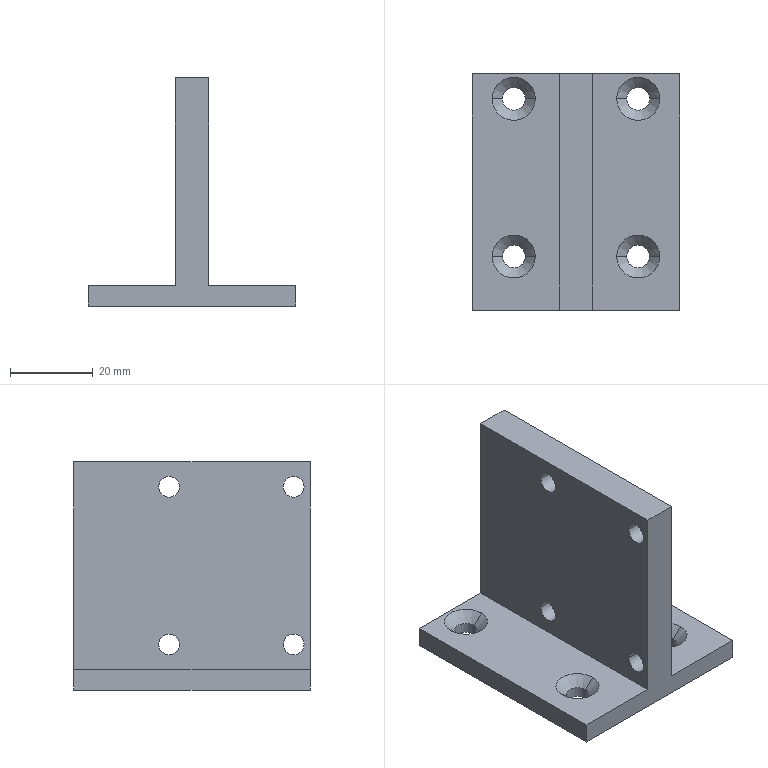Part | 1 solid | 34 faces | box 50 x 57 x 55 mm | volume 35677 mm3 | cylinder 16 | plane 10 | cone 8 | commonest cylinder face diameters 5 x8 5.5 x8
STEP:
#1=CARTESIAN_POINT('',(7.25,41.,2.55));
#2=VERTEX_POINT('',#1);
#3=CARTESIAN_POINT('',(12.75,41.,2.55));
#4=VERTEX_POINT('',#3);
#5=CARTESIAN_POINT('',(10.,41.,2.55));
#6=DIRECTION('',(0.,0.,1.));
#7=DIRECTION('',(1.,0.,0.));
#8=AXIS2_PLACEMENT_3D('',#5,#6,#7);
#9=CIRCLE('',#8,2.75);
#10=EDGE_CURVE('',#2,#4,#9,.T.);
#11=ORIENTED_EDGE('',*,*,#10,.F.);
#12=CARTESIAN_POINT('',(4.8,41.,5.));
#13=VERTEX_POINT('',#12);
#14=CARTESIAN_POINT('',(4.8,41.,5.));
#15=DIRECTION('',(-0.7071,0.,0.7071));
#16=VECTOR('',#15,1000.);
#17=LINE('',#14,#16);
#18=EDGE_CURVE('',#2,#13,#17,.T.);
#19=ORIENTED_EDGE('',*,*,#18,.T.);
#20=CARTESIAN_POINT('',(15.2,41.,5.));
#21=VERTEX_POINT('',#20);
#22=CARTESIAN_POINT('',(10.,41.,5.));
#23=DIRECTION('',(0.,0.,1.));
#24=DIRECTION('',(1.,0.,0.));
#25=AXIS2_PLACEMENT_3D('',#22,#23,#24);
#26=CIRCLE('',#25,5.2);
#27=EDGE_CURVE('',#13,#21,#26,.T.);
#28=ORIENTED_EDGE('',*,*,#27,.T.);
#29=CARTESIAN_POINT('',(15.2,41.,5.));
#30=DIRECTION('',(0.7071,0.,0.7071));
#31=VECTOR('',#30,1000.);
#32=LINE('',#29,#31);
#33=EDGE_CURVE('',#4,#21,#32,.T.);
#34=ORIENTED_EDGE('',*,*,#33,.F.);
#35=EDGE_LOOP('',(#11,#19,#28,#34));
#36=FACE_OUTER_BOUND('',#35,.T.);
#37=CARTESIAN_POINT('',(10.,41.,5.));
#38=DIRECTION('',(0.,0.,1.));
#39=DIRECTION('',(1.,0.,0.));
#40=AXIS2_PLACEMENT_3D('',#37,#38,#39);
#41=CONICAL_SURFACE('',#40,5.2,0.7854);
#42=ADVANCED_FACE('',(#36),#41,.F.);
#43=CARTESIAN_POINT('',(7.25,41.,0.));
#44=VERTEX_POINT('',#43);
#45=CARTESIAN_POINT('',(12.75,41.,0.));
#46=VERTEX_POINT('',#45);
#47=CARTESIAN_POINT('',(10.,41.,0.));
#48=DIRECTION('',(0.,0.,1.));
#49=DIRECTION('',(1.,0.,0.));
#50=AXIS2_PLACEMENT_3D('',#47,#48,#49);
#51=CIRCLE('',#50,2.75);
#52=EDGE_CURVE('',#44,#46,#51,.T.);
#53=ORIENTED_EDGE('',*,*,#52,.F.);
#54=CARTESIAN_POINT('',(7.25,41.,5.));
#55=DIRECTION('',(0.,0.,1.));
#56=VECTOR('',#55,1000.);
#57=LINE('',#54,#56);
#58=EDGE_CURVE('',#44,#2,#57,.T.);
#59=ORIENTED_EDGE('',*,*,#58,.T.);
#60=ORIENTED_EDGE('',*,*,#10,.T.);
#61=CARTESIAN_POINT('',(12.75,41.,5.));
#62=DIRECTION('',(0.,0.,1.));
#63=VECTOR('',#62,1000.);
#64=LINE('',#61,#63);
#65=EDGE_CURVE('',#46,#4,#64,.T.);
#66=ORIENTED_EDGE('',*,*,#65,.F.);
#67=EDGE_LOOP('',(#53,#59,#60,#66));
#68=FACE_OUTER_BOUND('',#67,.T.);
#69=CARTESIAN_POINT('',(10.,41.,5.));
#70=DIRECTION('',(0.,0.,1.));
#71=DIRECTION('',(1.,0.,0.));
#72=AXIS2_PLACEMENT_3D('',#69,#70,#71);
#73=CYLINDRICAL_SURFACE('',#72,2.75);
#74=ADVANCED_FACE('',(#68),#73,.F.);
#75=CARTESIAN_POINT('',(7.25,3.,2.55));
#76=VERTEX_POINT('',#75);
#77=CARTESIAN_POINT('',(12.75,3.,2.55));
#78=VERTEX_POINT('',#77);
#79=CARTESIAN_POINT('',(10.,3.,2.55));
#80=DIRECTION('',(0.,0.,1.));
#81=DIRECTION('',(1.,0.,0.));
#82=AXIS2_PLACEMENT_3D('',#79,#80,#81);
#83=CIRCLE('',#82,2.75);
#84=EDGE_CURVE('',#76,#78,#83,.T.);
#85=ORIENTED_EDGE('',*,*,#84,.F.);
#86=CARTESIAN_POINT('',(4.8,3.,5.));
#87=VERTEX_POINT('',#86);
#88=CARTESIAN_POINT('',(4.8,3.,5.));
#89=DIRECTION('',(-0.7071,0.,0.7071));
#90=VECTOR('',#89,1000.);
#91=LINE('',#88,#90);
#92=EDGE_CURVE('',#76,#87,#91,.T.);
#93=ORIENTED_EDGE('',*,*,#92,.T.);
#94=CARTESIAN_POINT('',(15.2,3.,5.));
#95=VERTEX_POINT('',#94);
#96=CARTESIAN_POINT('',(10.,3.,5.));
#97=DIRECTION('',(0.,0.,1.));
#98=DIRECTION('',(1.,0.,0.));
#99=AXIS2_PLACEMENT_3D('',#96,#97,#98);
#100=CIRCLE('',#99,5.2);
#101=EDGE_CURVE('',#87,#95,#100,.T.);
#102=ORIENTED_EDGE('',*,*,#101,.T.);
#103=CARTESIAN_POINT('',(15.2,3.,5.));
#104=DIRECTION('',(0.7071,0.,0.7071));
#105=VECTOR('',#104,1000.);
#106=LINE('',#103,#105);
#107=EDGE_CURVE('',#78,#95,#106,.T.);
#108=ORIENTED_EDGE('',*,*,#107,.F.);
#109=EDGE_LOOP('',(#85,#93,#102,#108));
#110=FACE_OUTER_BOUND('',#109,.T.);
#111=CARTESIAN_POINT('',(10.,3.,5.));
#112=DIRECTION('',(0.,0.,1.));
#113=DIRECTION('',(1.,0.,0.));
#114=AXIS2_PLACEMENT_3D('',#111,#112,#113);
#115=CONICAL_SURFACE('',#114,5.2,0.7854);
#116=ADVANCED_FACE('',(#110),#115,.F.);
#117=CARTESIAN_POINT('',(7.25,3.,0.));
#118=VERTEX_POINT('',#117);
#119=CARTESIAN_POINT('',(12.75,3.,0.));
#120=VERTEX_POINT('',#119);
#121=CARTESIAN_POINT('',(10.,3.,0.));
#122=DIRECTION('',(0.,0.,1.));
#123=DIRECTION('',(1.,0.,0.));
#124=AXIS2_PLACEMENT_3D('',#121,#122,#123);
#125=CIRCLE('',#124,2.75);
#126=EDGE_CURVE('',#118,#120,#125,.T.);
#127=ORIENTED_EDGE('',*,*,#126,.F.);
#128=CARTESIAN_POINT('',(7.25,3.,5.));
#129=DIRECTION('',(0.,0.,1.));
#130=VECTOR('',#129,1000.);
#131=LINE('',#128,#130);
#132=EDGE_CURVE('',#118,#76,#131,.T.);
#133=ORIENTED_EDGE('',*,*,#132,.T.);
#134=ORIENTED_EDGE('',*,*,#84,.T.);
#135=CARTESIAN_POINT('',(12.75,3.,5.));
#136=DIRECTION('',(0.,0.,1.));
#137=VECTOR('',#136,1000.);
#138=LINE('',#135,#137);
#139=EDGE_CURVE('',#120,#78,#138,.T.);
#140=ORIENTED_EDGE('',*,*,#139,.F.);
#141=EDGE_LOOP('',(#127,#133,#134,#140));
#142=FACE_OUTER_BOUND('',#141,.T.);
#143=CARTESIAN_POINT('',(10.,3.,5.));
#144=DIRECTION('',(0.,0.,1.));
#145=DIRECTION('',(1.,0.,0.));
#146=AXIS2_PLACEMENT_3D('',#143,#144,#145);
#147=CYLINDRICAL_SURFACE('',#146,2.75);
#148=ADVANCED_FACE('',(#142),#147,.F.);
#149=CARTESIAN_POINT('',(37.25,41.,2.55));
#150=VERTEX_POINT('',#149);
#151=CARTESIAN_POINT('',(42.75,41.,2.55));
#152=VERTEX_POINT('',#151);
#153=CARTESIAN_POINT('',(40.,41.,2.55));
#154=DIRECTION('',(0.,0.,1.));
#155=DIRECTION('',(1.,0.,0.));
#156=AXIS2_PLACEMENT_3D('',#153,#154,#155);
#157=CIRCLE('',#156,2.75);
#158=EDGE_CURVE('',#150,#152,#157,.T.);
#159=ORIENTED_EDGE('',*,*,#158,.F.);
#160=CARTESIAN_POINT('',(34.8,41.,5.));
#161=VERTEX_POINT('',#160);
#162=CARTESIAN_POINT('',(34.8,41.,5.));
#163=DIRECTION('',(-0.7071,0.,0.7071));
#164=VECTOR('',#163,1000.);
#165=LINE('',#162,#164);
#166=EDGE_CURVE('',#150,#161,#165,.T.);
#167=ORIENTED_EDGE('',*,*,#166,.T.);
#168=CARTESIAN_POINT('',(45.2,41.,5.));
#169=VERTEX_POINT('',#168);
#170=CARTESIAN_POINT('',(40.,41.,5.));
#171=DIRECTION('',(0.,0.,1.));
#172=DIRECTION('',(1.,0.,0.));
#173=AXIS2_PLACEMENT_3D('',#170,#171,#172);
#174=CIRCLE('',#173,5.2);
#175=EDGE_CURVE('',#161,#169,#174,.T.);
#176=ORIENTED_EDGE('',*,*,#175,.T.);
#177=CARTESIAN_POINT('',(45.2,41.,5.));
#178=DIRECTION('',(0.7071,0.,0.7071));
#179=VECTOR('',#178,1000.);
#180=LINE('',#177,#179);
#181=EDGE_CURVE('',#152,#169,#180,.T.);
#182=ORIENTED_EDGE('',*,*,#181,.F.);
#183=EDGE_LOOP('',(#159,#167,#176,#182));
#184=FACE_OUTER_BOUND('',#183,.T.);
#185=CARTESIAN_POINT('',(40.,41.,5.));
#186=DIRECTION('',(0.,0.,1.));
#187=DIRECTION('',(1.,0.,0.));
#188=AXIS2_PLACEMENT_3D('',#185,#186,#187);
#189=CONICAL_SURFACE('',#188,5.2,0.7854);
#190=ADVANCED_FACE('',(#184),#189,.F.);
#191=CARTESIAN_POINT('',(37.25,41.,0.));
#192=VERTEX_POINT('',#191);
#193=CARTESIAN_POINT('',(42.75,41.,0.));
#194=VERTEX_POINT('',#193);
#195=CARTESIAN_POINT('',(40.,41.,0.));
#196=DIRECTION('',(0.,0.,1.));
#197=DIRECTION('',(1.,0.,0.));
#198=AXIS2_PLACEMENT_3D('',#195,#196,#197);
#199=CIRCLE('',#198,2.75);
#200=EDGE_CURVE('',#192,#194,#199,.T.);
#201=ORIENTED_EDGE('',*,*,#200,.F.);
#202=CARTESIAN_POINT('',(37.25,41.,5.));
#203=DIRECTION('',(0.,0.,1.));
#204=VECTOR('',#203,1000.);
#205=LINE('',#202,#204);
#206=EDGE_CURVE('',#192,#150,#205,.T.);
#207=ORIENTED_EDGE('',*,*,#206,.T.);
#208=ORIENTED_EDGE('',*,*,#158,.T.);
#209=CARTESIAN_POINT('',(42.75,41.,5.));
#210=DIRECTION('',(0.,0.,1.));
#211=VECTOR('',#210,1000.);
#212=LINE('',#209,#211);
#213=EDGE_CURVE('',#194,#152,#212,.T.);
#214=ORIENTED_EDGE('',*,*,#213,.F.);
#215=EDGE_LOOP('',(#201,#207,#208,#214));
#216=FACE_OUTER_BOUND('',#215,.T.);
#217=CARTESIAN_POINT('',(40.,41.,5.));
#218=DIRECTION('',(0.,0.,1.));
#219=DIRECTION('',(1.,0.,0.));
#220=AXIS2_PLACEMENT_3D('',#217,#218,#219);
#221=CYLINDRICAL_SURFACE('',#220,2.75);
#222=ADVANCED_FACE('',(#216),#221,.F.);
#223=CARTESIAN_POINT('',(37.25,3.,2.55));
#224=VERTEX_POINT('',#223);
#225=CARTESIAN_POINT('',(42.75,3.,2.55));
#226=VERTEX_POINT('',#225);
#227=CARTESIAN_POINT('',(40.,3.,2.55));
#228=DIRECTION('',(0.,0.,1.));
#229=DIRECTION('',(1.,0.,0.));
#230=AXIS2_PLACEMENT_3D('',#227,#228,#229);
#231=CIRCLE('',#230,2.75);
#232=EDGE_CURVE('',#224,#226,#231,.T.);
#233=ORIENTED_EDGE('',*,*,#232,.F.);
#234=CARTESIAN_POINT('',(34.8,3.,5.));
#235=VERTEX_POINT('',#234);
#236=CARTESIAN_POINT('',(34.8,3.,5.));
#237=DIRECTION('',(-0.7071,0.,0.7071));
#238=VECTOR('',#237,1000.);
#239=LINE('',#236,#238);
#240=EDGE_CURVE('',#224,#235,#239,.T.);
#241=ORIENTED_EDGE('',*,*,#240,.T.);
#242=CARTESIAN_POINT('',(45.2,3.,5.));
#243=VERTEX_POINT('',#242);
#244=CARTESIAN_POINT('',(40.,3.,5.));
#245=DIRECTION('',(0.,0.,1.));
#246=DIRECTION('',(1.,0.,0.));
#247=AXIS2_PLACEMENT_3D('',#244,#245,#246);
#248=CIRCLE('',#247,5.2);
#249=EDGE_CURVE('',#235,#243,#248,.T.);
#250=ORIENTED_EDGE('',*,*,#249,.T.);
#251=CARTESIAN_POINT('',(45.2,3.,5.));
#252=DIRECTION('',(0.7071,0.,0.7071));
#253=VECTOR('',#252,1000.);
#254=LINE('',#251,#253);
#255=EDGE_CURVE('',#226,#243,#254,.T.);
#256=ORIENTED_EDGE('',*,*,#255,.F.);
#257=EDGE_LOOP('',(#233,#241,#250,#256));
#258=FACE_OUTER_BOUND('',#257,.T.);
#259=CARTESIAN_POINT('',(40.,3.,5.));
#260=DIRECTION('',(0.,0.,1.));
#261=DIRECTION('',(1.,0.,0.));
#262=AXIS2_PLACEMENT_3D('',#259,#260,#261);
#263=CONICAL_SURFACE('',#262,5.2,0.7854);
#264=ADVANCED_FACE('',(#258),#263,.F.);
#265=CARTESIAN_POINT('',(37.25,3.,0.));
#266=VERTEX_POINT('',#265);
#267=CARTESIAN_POINT('',(42.75,3.,0.));
#268=VERTEX_POINT('',#267);
#269=CARTESIAN_POINT('',(40.,3.,0.));
#270=DIRECTION('',(0.,0.,1.));
#271=DIRECTION('',(1.,0.,0.));
#272=AXIS2_PLACEMENT_3D('',#269,#270,#271);
#273=CIRCLE('',#272,2.75);
#274=EDGE_CURVE('',#266,#268,#273,.T.);
#275=ORIENTED_EDGE('',*,*,#274,.F.);
#276=CARTESIAN_POINT('',(37.25,3.,5.));
#277=DIRECTION('',(0.,0.,1.));
#278=VECTOR('',#277,1000.);
#279=LINE('',#276,#278);
#280=EDGE_CURVE('',#266,#224,#279,.T.);
#281=ORIENTED_EDGE('',*,*,#280,.T.);
#282=ORIENTED_EDGE('',*,*,#232,.T.);
#283=CARTESIAN_POINT('',(42.75,3.,5.));
#284=DIRECTION('',(0.,0.,1.));
#285=VECTOR('',#284,1000.);
#286=LINE('',#283,#285);
#287=EDGE_CURVE('',#268,#226,#286,.T.);
#288=ORIENTED_EDGE('',*,*,#287,.F.);
#289=EDGE_LOOP('',(#275,#281,#282,#288));
#290=FACE_OUTER_BOUND('',#289,.T.);
#291=CARTESIAN_POINT('',(40.,3.,5.));
#292=DIRECTION('',(0.,0.,1.));
#293=DIRECTION('',(1.,0.,0.));
#294=AXIS2_PLACEMENT_3D('',#291,#292,#293);
#295=CYLINDRICAL_SURFACE('',#294,2.75);
#296=ADVANCED_FACE('',(#290),#295,.F.);
#297=CARTESIAN_POINT('',(29.,-3.5,49.));
#298=VERTEX_POINT('',#297);
#299=CARTESIAN_POINT('',(29.,-8.5,49.));
#300=VERTEX_POINT('',#299);
#301=CARTESIAN_POINT('',(29.,-6.,49.));
#302=DIRECTION('',(-1.,0.,0.));
#303=DIRECTION('',(0.,-1.,0.));
#304=AXIS2_PLACEMENT_3D('',#301,#302,#303);
#305=CIRCLE('',#304,2.5);
#306=EDGE_CURVE('',#298,#300,#305,.T.);
#307=ORIENTED_EDGE('',*,*,#306,.F.);
#308=CARTESIAN_POINT('',(21.,-3.5,49.));
#309=VERTEX_POINT('',#308);
#310=CARTESIAN_POINT('',(50.,-3.5,49.));
#311=DIRECTION('',(-1.,0.,0.));
#312=VECTOR('',#311,1000.);
#313=LINE('',#310,#312);
#314=EDGE_CURVE('',#298,#309,#313,.T.);
#315=ORIENTED_EDGE('',*,*,#314,.T.);
#316=CARTESIAN_POINT('',(21.,-8.5,49.));
#317=VERTEX_POINT('',#316);
#318=CARTESIAN_POINT('',(21.,-6.,49.));
#319=DIRECTION('',(-1.,0.,0.));
#320=DIRECTION('',(0.,-1.,0.));
#321=AXIS2_PLACEMENT_3D('',#318,#319,#320);
#322=CIRCLE('',#321,2.5);
#323=EDGE_CURVE('',#309,#317,#322,.T.);
#324=ORIENTED_EDGE('',*,*,#323,.T.);
#325=CARTESIAN_POINT('',(50.,-8.5,49.));
#326=DIRECTION('',(-1.,0.,0.));
#327=VECTOR('',#326,1000.);
#328=LINE('',#325,#327);
#329=EDGE_CURVE('',#300,#317,#328,.T.);
#330=ORIENTED_EDGE('',*,*,#329,.F.);
#331=EDGE_LOOP('',(#307,#315,#324,#330));
#332=FACE_OUTER_BOUND('',#331,.T.);
#333=CARTESIAN_POINT('',(50.,-6.,49.));
#334=DIRECTION('',(-1.,0.,0.));
#335=DIRECTION('',(0.,-1.,0.));
#336=AXIS2_PLACEMENT_3D('',#333,#334,#335);
#337=CYLINDRICAL_SURFACE('',#336,2.5);
#338=ADVANCED_FACE('',(#332),#337,.F.);
#339=CARTESIAN_POINT('',(29.,-3.5,11.));
#340=VERTEX_POINT('',#339);
#341=CARTESIAN_POINT('',(29.,-8.5,11.));
#342=VERTEX_POINT('',#341);
#343=CARTESIAN_POINT('',(29.,-6.,11.));
#344=DIRECTION('',(-1.,0.,0.));
#345=DIRECTION('',(0.,-1.,0.));
#346=AXIS2_PLACEMENT_3D('',#343,#344,#345);
#347=CIRCLE('',#346,2.5);
#348=EDGE_CURVE('',#340,#342,#347,.T.);
#349=ORIENTED_EDGE('',*,*,#348,.F.);
#350=CARTESIAN_POINT('',(21.,-3.5,11.));
#351=VERTEX_POINT('',#350);
#352=CARTESIAN_POINT('',(50.,-3.5,11.));
#353=DIRECTION('',(-1.,0.,0.));
#354=VECTOR('',#353,1000.);
#355=LINE('',#352,#354);
#356=EDGE_CURVE('',#340,#351,#355,.T.);
#357=ORIENTED_EDGE('',*,*,#356,.T.);
#358=CARTESIAN_POINT('',(21.,-8.5,11.));
#359=VERTEX_POINT('',#358);
#360=CARTESIAN_POINT('',(21.,-6.,11.));
#361=DIRECTION('',(-1.,0.,0.));
#362=DIRECTION('',(0.,-1.,0.));
#363=AXIS2_PLACEMENT_3D('',#360,#361,#362);
#364=CIRCLE('',#363,2.5);
#365=EDGE_CURVE('',#351,#359,#364,.T.);
#366=ORIENTED_EDGE('',*,*,#365,.T.);
#367=CARTESIAN_POINT('',(50.,-8.5,11.));
#368=DIRECTION('',(-1.,0.,0.));
#369=VECTOR('',#368,1000.);
#370=LINE('',#367,#369);
#371=EDGE_CURVE('',#342,#359,#370,.T.);
#372=ORIENTED_EDGE('',*,*,#371,.F.);
#373=EDGE_LOOP('',(#349,#357,#366,#372));
#374=FACE_OUTER_BOUND('',#373,.T.);
#375=CARTESIAN_POINT('',(50.,-6.,11.));
#376=DIRECTION('',(-1.,0.,0.));
#377=DIRECTION('',(0.,-1.,0.));
#378=AXIS2_PLACEMENT_3D('',#375,#376,#377);
#379=CYLINDRICAL_SURFACE('',#378,2.5);
#380=ADVANCED_FACE('',(#374),#379,.F.);
#381=CARTESIAN_POINT('',(29.,26.5,49.));
#382=VERTEX_POINT('',#381);
#383=CARTESIAN_POINT('',(29.,21.5,49.));
#384=VERTEX_POINT('',#383);
#385=CARTESIAN_POINT('',(29.,24.,49.));
#386=DIRECTION('',(-1.,0.,0.));
#387=DIRECTION('',(0.,-1.,0.));
#388=AXIS2_PLACEMENT_3D('',#385,#386,#387);
#389=CIRCLE('',#388,2.5);
#390=EDGE_CURVE('',#382,#384,#389,.T.);
#391=ORIENTED_EDGE('',*,*,#390,.F.);
#392=CARTESIAN_POINT('',(21.,26.5,49.));
#393=VERTEX_POINT('',#392);
#394=CARTESIAN_POINT('',(50.,26.5,49.));
#395=DIRECTION('',(-1.,0.,0.));
#396=VECTOR('',#395,1000.);
#397=LINE('',#394,#396);
#398=EDGE_CURVE('',#382,#393,#397,.T.);
#399=ORIENTED_EDGE('',*,*,#398,.T.);
#400=CARTESIAN_POINT('',(21.,21.5,49.));
#401=VERTEX_POINT('',#400);
#402=CARTESIAN_POINT('',(21.,24.,49.));
#403=DIRECTION('',(-1.,0.,0.));
#404=DIRECTION('',(0.,-1.,0.));
#405=AXIS2_PLACEMENT_3D('',#402,#403,#404);
#406=CIRCLE('',#405,2.5);
#407=EDGE_CURVE('',#393,#401,#406,.T.);
#408=ORIENTED_EDGE('',*,*,#407,.T.);
#409=CARTESIAN_POINT('',(50.,21.5,49.));
#410=DIRECTION('',(-1.,0.,0.));
#411=VECTOR('',#410,1000.);
#412=LINE('',#409,#411);
#413=EDGE_CURVE('',#384,#401,#412,.T.);
#414=ORIENTED_EDGE('',*,*,#413,.F.);
#415=EDGE_LOOP('',(#391,#399,#408,#414));
#416=FACE_OUTER_BOUND('',#415,.T.);
#417=CARTESIAN_POINT('',(50.,24.,49.));
#418=DIRECTION('',(-1.,0.,0.));
#419=DIRECTION('',(0.,-1.,0.));
#420=AXIS2_PLACEMENT_3D('',#417,#418,#419);
#421=CYLINDRICAL_SURFACE('',#420,2.5);
#422=ADVANCED_FACE('',(#416),#421,.F.);
#423=CARTESIAN_POINT('',(29.,26.5,11.));
#424=VERTEX_POINT('',#423);
#425=CARTESIAN_POINT('',(29.,21.5,11.));
#426=VERTEX_POINT('',#425);
#427=CARTESIAN_POINT('',(29.,24.,11.));
#428=DIRECTION('',(-1.,0.,0.));
#429=DIRECTION('',(0.,-1.,0.));
#430=AXIS2_PLACEMENT_3D('',#427,#428,#429);
#431=CIRCLE('',#430,2.5);
#432=EDGE_CURVE('',#424,#426,#431,.T.);
#433=ORIENTED_EDGE('',*,*,#432,.F.);
#434=CARTESIAN_POINT('',(21.,26.5,11.));
#435=VERTEX_POINT('',#434);
#436=CARTESIAN_POINT('',(50.,26.5,11.));
#437=DIRECTION('',(-1.,0.,0.));
#438=VECTOR('',#437,1000.);
#439=LINE('',#436,#438);
#440=EDGE_CURVE('',#424,#435,#439,.T.);
#441=ORIENTED_EDGE('',*,*,#440,.T.);
#442=CARTESIAN_POINT('',(21.,21.5,11.));
#443=VERTEX_POINT('',#442);
#444=CARTESIAN_POINT('',(21.,24.,11.));
#445=DIRECTION('',(-1.,0.,0.));
#446=DIRECTION('',(0.,-1.,0.));
#447=AXIS2_PLACEMENT_3D('',#444,#445,#446);
#448=CIRCLE('',#447,2.5);
#449=EDGE_CURVE('',#435,#443,#448,.T.);
#450=ORIENTED_EDGE('',*,*,#449,.T.);
#451=CARTESIAN_POINT('',(50.,21.5,11.));
#452=DIRECTION('',(-1.,0.,0.));
#453=VECTOR('',#452,1000.);
#454=LINE('',#451,#453);
#455=EDGE_CURVE('',#426,#443,#454,.T.);
#456=ORIENTED_EDGE('',*,*,#455,.F.);
#457=EDGE_LOOP('',(#433,#441,#450,#456));
#458=FACE_OUTER_BOUND('',#457,.T.);
#459=CARTESIAN_POINT('',(50.,24.,11.));
#460=DIRECTION('',(-1.,0.,0.));
#461=DIRECTION('',(0.,-1.,0.));
#462=AXIS2_PLACEMENT_3D('',#459,#460,#461);
#463=CYLINDRICAL_SURFACE('',#462,2.5);
#464=ADVANCED_FACE('',(#458),#463,.F.);
#465=CARTESIAN_POINT('',(10.,41.,5.));
#466=DIRECTION('',(0.,0.,1.));
#467=DIRECTION('',(1.,0.,0.));
#468=AXIS2_PLACEMENT_3D('',#465,#466,#467);
#469=CIRCLE('',#468,5.2);
#470=EDGE_CURVE('',#21,#13,#469,.T.);
#471=ORIENTED_EDGE('',*,*,#470,.F.);
#472=ORIENTED_EDGE('',*,*,#27,.F.);
#473=EDGE_LOOP('',(#471,#472));
#474=FACE_BOUND('',#473,.T.);
#475=CARTESIAN_POINT('',(10.,3.,5.));
#476=DIRECTION('',(0.,0.,1.));
#477=DIRECTION('',(1.,0.,0.));
#478=AXIS2_PLACEMENT_3D('',#475,#476,#477);
#479=CIRCLE('',#478,5.2);
#480=EDGE_CURVE('',#95,#87,#479,.T.);
#481=ORIENTED_EDGE('',*,*,#480,.F.);
#482=ORIENTED_EDGE('',*,*,#101,.F.);
#483=EDGE_LOOP('',(#481,#482));
#484=FACE_BOUND('',#483,.T.);
#485=CARTESIAN_POINT('',(21.,47.,5.));
#486=VERTEX_POINT('',#485);
#487=CARTESIAN_POINT('',(21.,-10.,5.));
#488=VERTEX_POINT('',#487);
#489=CARTESIAN_POINT('',(21.,47.,5.));
#490=DIRECTION('',(0.,-1.,0.));
#491=VECTOR('',#490,1000.);
#492=LINE('',#489,#491);
#493=EDGE_CURVE('',#486,#488,#492,.T.);
#494=ORIENTED_EDGE('',*,*,#493,.F.);
#495=CARTESIAN_POINT('',(0.,47.,5.));
#496=VERTEX_POINT('',#495);
#497=CARTESIAN_POINT('',(0.,47.,5.));
#498=DIRECTION('',(-1.,0.,0.));
#499=VECTOR('',#498,1000.);
#500=LINE('',#497,#499);
#501=EDGE_CURVE('',#486,#496,#500,.T.);
#502=ORIENTED_EDGE('',*,*,#501,.T.);
#503=CARTESIAN_POINT('',(0.,-10.,5.));
#504=VERTEX_POINT('',#503);
#505=CARTESIAN_POINT('',(0.,0.,5.));
#506=DIRECTION('',(0.,-1.,0.));
#507=VECTOR('',#506,1000.);
#508=LINE('',#505,#507);
#509=EDGE_CURVE('',#496,#504,#508,.T.);
#510=ORIENTED_EDGE('',*,*,#509,.T.);
#511=CARTESIAN_POINT('',(21.,-10.,5.));
#512=DIRECTION('',(-1.,0.,0.));
#513=VECTOR('',#512,1000.);
#514=LINE('',#511,#513);
#515=EDGE_CURVE('',#488,#504,#514,.T.);
#516=ORIENTED_EDGE('',*,*,#515,.F.);
#517=EDGE_LOOP('',(#494,#502,#510,#516));
#518=FACE_OUTER_BOUND('',#517,.T.);
#519=CARTESIAN_POINT('',(0.,0.,5.));
#520=DIRECTION('',(0.,0.,-1.));
#521=DIRECTION('',(-1.,0.,0.));
#522=AXIS2_PLACEMENT_3D('',#519,#520,#521);
#523=PLANE('',#522);
#524=ADVANCED_FACE('',(#474,#484,#518),#523,.F.);
#525=CARTESIAN_POINT('',(40.,41.,5.));
#526=DIRECTION('',(0.,0.,1.));
#527=DIRECTION('',(1.,0.,0.));
#528=AXIS2_PLACEMENT_3D('',#525,#526,#527);
#529=CIRCLE('',#528,5.2);
#530=EDGE_CURVE('',#169,#161,#529,.T.);
#531=ORIENTED_EDGE('',*,*,#530,.F.);
#532=ORIENTED_EDGE('',*,*,#175,.F.);
#533=EDGE_LOOP('',(#531,#532));
#534=FACE_BOUND('',#533,.T.);
#535=CARTESIAN_POINT('',(40.,3.,5.));
#536=DIRECTION('',(0.,0.,1.));
#537=DIRECTION('',(1.,0.,0.));
#538=AXIS2_PLACEMENT_3D('',#535,#536,#537);
#539=CIRCLE('',#538,5.2);
#540=EDGE_CURVE('',#243,#235,#539,.T.);
#541=ORIENTED_EDGE('',*,*,#540,.F.);
#542=ORIENTED_EDGE('',*,*,#249,.F.);
#543=EDGE_LOOP('',(#541,#542));
#544=FACE_BOUND('',#543,.T.);
#545=CARTESIAN_POINT('',(29.,-10.,5.));
#546=VERTEX_POINT('',#545);
#547=CARTESIAN_POINT('',(29.,47.,5.));
#548=VERTEX_POINT('',#547);
#549=CARTESIAN_POINT('',(29.,47.,5.));
#550=DIRECTION('',(0.,1.,0.));
#551=VECTOR('',#550,1000.);
#552=LINE('',#549,#551);
#553=EDGE_CURVE('',#546,#548,#552,.T.);
#554=ORIENTED_EDGE('',*,*,#553,.F.);
#555=CARTESIAN_POINT('',(50.,-10.,5.));
#556=VERTEX_POINT('',#555);
#557=CARTESIAN_POINT('',(50.,-10.,5.));
#558=DIRECTION('',(-1.,0.,0.));
#559=VECTOR('',#558,1000.);
#560=LINE('',#557,#559);
#561=EDGE_CURVE('',#556,#546,#560,.T.);
#562=ORIENTED_EDGE('',*,*,#561,.F.);
#563=CARTESIAN_POINT('',(50.,47.,5.));
#564=VERTEX_POINT('',#563);
#565=CARTESIAN_POINT('',(50.,0.,5.));
#566=DIRECTION('',(0.,1.,0.));
#567=VECTOR('',#566,1000.);
#568=LINE('',#565,#567);
#569=EDGE_CURVE('',#556,#564,#568,.T.);
#570=ORIENTED_EDGE('',*,*,#569,.T.);
#571=CARTESIAN_POINT('',(0.,47.,5.));
#572=DIRECTION('',(-1.,0.,0.));
#573=VECTOR('',#572,1000.);
#574=LINE('',#571,#573);
#575=EDGE_CURVE('',#564,#548,#574,.T.);
#576=ORIENTED_EDGE('',*,*,#575,.T.);
#577=EDGE_LOOP('',(#554,#562,#570,#576));
#578=FACE_OUTER_BOUND('',#577,.T.);
#579=CARTESIAN_POINT('',(0.,0.,5.));
#580=DIRECTION('',(0.,0.,-1.));
#581=DIRECTION('',(-1.,0.,0.));
#582=AXIS2_PLACEMENT_3D('',#579,#580,#581);
#583=PLANE('',#582);
#584=ADVANCED_FACE('',(#534,#544,#578),#583,.F.);
#585=CARTESIAN_POINT('',(0.,47.,0.));
#586=VERTEX_POINT('',#585);
#587=CARTESIAN_POINT('',(0.,-10.,0.));
#588=VERTEX_POINT('',#587);
#589=CARTESIAN_POINT('',(0.,0.,0.));
#590=DIRECTION('',(0.,-1.,0.));
#591=VECTOR('',#590,1000.);
#592=LINE('',#589,#591);
#593=EDGE_CURVE('',#586,#588,#592,.T.);
#594=ORIENTED_EDGE('',*,*,#593,.T.);
#595=CARTESIAN_POINT('',(0.,-10.,5.));
#596=DIRECTION('',(0.,0.,-1.));
#597=VECTOR('',#596,1000.);
#598=LINE('',#595,#597);
#599=EDGE_CURVE('',#504,#588,#598,.T.);
#600=ORIENTED_EDGE('',*,*,#599,.F.);
#601=ORIENTED_EDGE('',*,*,#509,.F.);
#602=CARTESIAN_POINT('',(0.,47.,5.));
#603=DIRECTION('',(0.,0.,-1.));
#604=VECTOR('',#603,1000.);
#605=LINE('',#602,#604);
#606=EDGE_CURVE('',#496,#586,#605,.T.);
#607=ORIENTED_EDGE('',*,*,#606,.T.);
#608=EDGE_LOOP('',(#594,#600,#601,#607));
#609=FACE_OUTER_BOUND('',#608,.T.);
#610=CARTESIAN_POINT('',(0.,0.,5.));
#611=DIRECTION('',(1.,0.,0.));
#612=DIRECTION('',(0.,0.,-1.));
#613=AXIS2_PLACEMENT_3D('',#610,#611,#612);
#614=PLANE('',#613);
#615=ADVANCED_FACE('',(#609),#614,.F.);
#616=CARTESIAN_POINT('',(50.,-10.,0.));
#617=VERTEX_POINT('',#616);
#618=CARTESIAN_POINT('',(50.,47.,0.));
#619=VERTEX_POINT('',#618);
#620=CARTESIAN_POINT('',(50.,0.,0.));
#621=DIRECTION('',(0.,1.,0.));
#622=VECTOR('',#621,1000.);
#623=LINE('',#620,#622);
#624=EDGE_CURVE('',#617,#619,#623,.T.);
#625=ORIENTED_EDGE('',*,*,#624,.T.);
#626=CARTESIAN_POINT('',(50.,47.,5.));
#627=DIRECTION('',(0.,0.,-1.));
#628=VECTOR('',#627,1000.);
#629=LINE('',#626,#628);
#630=EDGE_CURVE('',#564,#619,#629,.T.);
#631=ORIENTED_EDGE('',*,*,#630,.F.);
#632=ORIENTED_EDGE('',*,*,#569,.F.);
#633=CARTESIAN_POINT('',(50.,-10.,0.));
#634=DIRECTION('',(0.,0.,1.));
#635=VECTOR('',#634,1000.);
#636=LINE('',#633,#635);
#637=EDGE_CURVE('',#617,#556,#636,.T.);
#638=ORIENTED_EDGE('',*,*,#637,.F.);
#639=EDGE_LOOP('',(#625,#631,#632,#638));
#640=FACE_OUTER_BOUND('',#639,.T.);
#641=CARTESIAN_POINT('',(50.,0.,5.));
#642=DIRECTION('',(-1.,0.,0.));
#643=DIRECTION('',(0.,0.,1.));
#644=AXIS2_PLACEMENT_3D('',#641,#642,#643);
#645=PLANE('',#644);
#646=ADVANCED_FACE('',(#640),#645,.F.);
#647=CARTESIAN_POINT('',(0.,47.,0.));
#648=DIRECTION('',(-1.,0.,0.));
#649=VECTOR('',#648,1000.);
#650=LINE('',#647,#649);
#651=EDGE_CURVE('',#619,#586,#650,.T.);
#652=ORIENTED_EDGE('',*,*,#651,.T.);
#653=ORIENTED_EDGE('',*,*,#606,.F.);
#654=ORIENTED_EDGE('',*,*,#501,.F.);
#655=CARTESIAN_POINT('',(21.,47.,55.));
#656=VERTEX_POINT('',#655);
#657=CARTESIAN_POINT('',(21.,47.,55.));
#658=DIRECTION('',(0.,0.,-1.));
#659=VECTOR('',#658,1000.);
#660=LINE('',#657,#659);
#661=EDGE_CURVE('',#656,#486,#660,.T.);
#662=ORIENTED_EDGE('',*,*,#661,.F.);
#663=CARTESIAN_POINT('',(29.,47.,55.));
#664=VERTEX_POINT('',#663);
#665=CARTESIAN_POINT('',(21.,47.,55.));
#666=DIRECTION('',(-1.,0.,0.));
#667=VECTOR('',#666,1000.);
#668=LINE('',#665,#667);
#669=EDGE_CURVE('',#664,#656,#668,.T.);
#670=ORIENTED_EDGE('',*,*,#669,.F.);
#671=CARTESIAN_POINT('',(29.,47.,55.));
#672=DIRECTION('',(0.,0.,-1.));
#673=VECTOR('',#672,1000.);
#674=LINE('',#671,#673);
#675=EDGE_CURVE('',#664,#548,#674,.T.);
#676=ORIENTED_EDGE('',*,*,#675,.T.);
#677=ORIENTED_EDGE('',*,*,#575,.F.);
#678=ORIENTED_EDGE('',*,*,#630,.T.);
#679=EDGE_LOOP('',(#652,#653,#654,#662,#670,#676,#677,#678));
#680=FACE_OUTER_BOUND('',#679,.T.);
#681=CARTESIAN_POINT('',(0.,47.,5.));
#682=DIRECTION('',(0.,-1.,0.));
#683=DIRECTION('',(0.,0.,-1.));
#684=AXIS2_PLACEMENT_3D('',#681,#682,#683);
#685=PLANE('',#684);
#686=ADVANCED_FACE('',(#680),#685,.F.);
#687=CARTESIAN_POINT('',(10.,41.,0.));
#688=DIRECTION('',(0.,0.,1.));
#689=DIRECTION('',(1.,0.,0.));
#690=AXIS2_PLACEMENT_3D('',#687,#688,#689);
#691=CIRCLE('',#690,2.75);
#692=EDGE_CURVE('',#46,#44,#691,.T.);
#693=ORIENTED_EDGE('',*,*,#692,.T.);
#694=ORIENTED_EDGE('',*,*,#52,.T.);
#695=EDGE_LOOP('',(#693,#694));
#696=FACE_BOUND('',#695,.T.);
#697=CARTESIAN_POINT('',(10.,3.,0.));
#698=DIRECTION('',(0.,0.,1.));
#699=DIRECTION('',(1.,0.,0.));
#700=AXIS2_PLACEMENT_3D('',#697,#698,#699);
#701=CIRCLE('',#700,2.75);
#702=EDGE_CURVE('',#120,#118,#701,.T.);
#703=ORIENTED_EDGE('',*,*,#702,.T.);
#704=ORIENTED_EDGE('',*,*,#126,.T.);
#705=EDGE_LOOP('',(#703,#704));
#706=FACE_BOUND('',#705,.T.);
#707=CARTESIAN_POINT('',(40.,41.,0.));
#708=DIRECTION('',(0.,0.,1.));
#709=DIRECTION('',(1.,0.,0.));
#710=AXIS2_PLACEMENT_3D('',#707,#708,#709);
#711=CIRCLE('',#710,2.75);
#712=EDGE_CURVE('',#194,#192,#711,.T.);
#713=ORIENTED_EDGE('',*,*,#712,.T.);
#714=ORIENTED_EDGE('',*,*,#200,.T.);
#715=EDGE_LOOP('',(#713,#714));
#716=FACE_BOUND('',#715,.T.);
#717=CARTESIAN_POINT('',(40.,3.,0.));
#718=DIRECTION('',(0.,0.,1.));
#719=DIRECTION('',(1.,0.,0.));
#720=AXIS2_PLACEMENT_3D('',#717,#718,#719);
#721=CIRCLE('',#720,2.75);
#722=EDGE_CURVE('',#268,#266,#721,.T.);
#723=ORIENTED_EDGE('',*,*,#722,.T.);
#724=ORIENTED_EDGE('',*,*,#274,.T.);
#725=EDGE_LOOP('',(#723,#724));
#726=FACE_BOUND('',#725,.T.);
#727=ORIENTED_EDGE('',*,*,#593,.F.);
#728=ORIENTED_EDGE('',*,*,#651,.F.);
#729=ORIENTED_EDGE('',*,*,#624,.F.);
#730=CARTESIAN_POINT('',(0.,-10.,0.));
#731=DIRECTION('',(1.,0.,0.));
#732=VECTOR('',#731,1000.);
#733=LINE('',#730,#732);
#734=EDGE_CURVE('',#588,#617,#733,.T.);
#735=ORIENTED_EDGE('',*,*,#734,.F.);
#736=EDGE_LOOP('',(#727,#728,#729,#735));
#737=FACE_OUTER_BOUND('',#736,.T.);
#738=CARTESIAN_POINT('',(0.,0.,0.));
#739=DIRECTION('',(0.,0.,-1.));
#740=DIRECTION('',(-1.,0.,0.));
#741=AXIS2_PLACEMENT_3D('',#738,#739,#740);
#742=PLANE('',#741);
#743=ADVANCED_FACE('',(#696,#706,#716,#726,#737),#742,.T.);
#744=CARTESIAN_POINT('',(21.,-6.,49.));
#745=DIRECTION('',(-1.,0.,0.));
#746=DIRECTION('',(0.,-1.,0.));
#747=AXIS2_PLACEMENT_3D('',#744,#745,#746);
#748=CIRCLE('',#747,2.5);
#749=EDGE_CURVE('',#317,#309,#748,.T.);
#750=ORIENTED_EDGE('',*,*,#749,.F.);
#751=ORIENTED_EDGE('',*,*,#323,.F.);
#752=EDGE_LOOP('',(#750,#751));
#753=FACE_BOUND('',#752,.T.);
#754=CARTESIAN_POINT('',(21.,-6.,11.));
#755=DIRECTION('',(-1.,0.,0.));
#756=DIRECTION('',(0.,-1.,0.));
#757=AXIS2_PLACEMENT_3D('',#754,#755,#756);
#758=CIRCLE('',#757,2.5);
#759=EDGE_CURVE('',#359,#351,#758,.T.);
#760=ORIENTED_EDGE('',*,*,#759,.F.);
#761=ORIENTED_EDGE('',*,*,#365,.F.);
#762=EDGE_LOOP('',(#760,#761));
#763=FACE_BOUND('',#762,.T.);
#764=CARTESIAN_POINT('',(21.,24.,49.));
#765=DIRECTION('',(-1.,0.,0.));
#766=DIRECTION('',(0.,-1.,0.));
#767=AXIS2_PLACEMENT_3D('',#764,#765,#766);
#768=CIRCLE('',#767,2.5);
#769=EDGE_CURVE('',#401,#393,#768,.T.);
#770=ORIENTED_EDGE('',*,*,#769,.F.);
#771=ORIENTED_EDGE('',*,*,#407,.F.);
#772=EDGE_LOOP('',(#770,#771));
#773=FACE_BOUND('',#772,.T.);
#774=CARTESIAN_POINT('',(21.,24.,11.));
#775=DIRECTION('',(-1.,0.,0.));
#776=DIRECTION('',(0.,-1.,0.));
#777=AXIS2_PLACEMENT_3D('',#774,#775,#776);
#778=CIRCLE('',#777,2.5);
#779=EDGE_CURVE('',#443,#435,#778,.T.);
#780=ORIENTED_EDGE('',*,*,#779,.F.);
#781=ORIENTED_EDGE('',*,*,#449,.F.);
#782=EDGE_LOOP('',(#780,#781));
#783=FACE_BOUND('',#782,.T.);
#784=ORIENTED_EDGE('',*,*,#493,.T.);
#785=CARTESIAN_POINT('',(21.,-10.,55.));
#786=VERTEX_POINT('',#785);
#787=CARTESIAN_POINT('',(21.,-10.,55.));
#788=DIRECTION('',(0.,0.,-1.));
#789=VECTOR('',#788,1000.);
#790=LINE('',#787,#789);
#791=EDGE_CURVE('',#786,#488,#790,.T.);
#792=ORIENTED_EDGE('',*,*,#791,.F.);
#793=CARTESIAN_POINT('',(21.,47.,55.));
#794=DIRECTION('',(0.,-1.,0.));
#795=VECTOR('',#794,1000.);
#796=LINE('',#793,#795);
#797=EDGE_CURVE('',#656,#786,#796,.T.);
#798=ORIENTED_EDGE('',*,*,#797,.F.);
#799=ORIENTED_EDGE('',*,*,#661,.T.);
#800=EDGE_LOOP('',(#784,#792,#798,#799));
#801=FACE_OUTER_BOUND('',#800,.T.);
#802=CARTESIAN_POINT('',(21.,47.,55.));
#803=DIRECTION('',(1.,0.,0.));
#804=DIRECTION('',(0.,1.,0.));
#805=AXIS2_PLACEMENT_3D('',#802,#803,#804);
#806=PLANE('',#805);
#807=ADVANCED_FACE('',(#753,#763,#773,#783,#801),#806,.F.);
#808=CARTESIAN_POINT('',(29.,-6.,49.));
#809=DIRECTION('',(-1.,0.,0.));
#810=DIRECTION('',(0.,-1.,0.));
#811=AXIS2_PLACEMENT_3D('',#808,#809,#810);
#812=CIRCLE('',#811,2.5);
#813=EDGE_CURVE('',#300,#298,#812,.T.);
#814=ORIENTED_EDGE('',*,*,#813,.T.);
#815=ORIENTED_EDGE('',*,*,#306,.T.);
#816=EDGE_LOOP('',(#814,#815));
#817=FACE_BOUND('',#816,.T.);
#818=CARTESIAN_POINT('',(29.,-6.,11.));
#819=DIRECTION('',(-1.,0.,0.));
#820=DIRECTION('',(0.,-1.,0.));
#821=AXIS2_PLACEMENT_3D('',#818,#819,#820);
#822=CIRCLE('',#821,2.5);
#823=EDGE_CURVE('',#342,#340,#822,.T.);
#824=ORIENTED_EDGE('',*,*,#823,.T.);
#825=ORIENTED_EDGE('',*,*,#348,.T.);
#826=EDGE_LOOP('',(#824,#825));
#827=FACE_BOUND('',#826,.T.);
#828=CARTESIAN_POINT('',(29.,24.,49.));
#829=DIRECTION('',(-1.,0.,0.));
#830=DIRECTION('',(0.,-1.,0.));
#831=AXIS2_PLACEMENT_3D('',#828,#829,#830);
#832=CIRCLE('',#831,2.5);
#833=EDGE_CURVE('',#384,#382,#832,.T.);
#834=ORIENTED_EDGE('',*,*,#833,.T.);
#835=ORIENTED_EDGE('',*,*,#390,.T.);
#836=EDGE_LOOP('',(#834,#835));
#837=FACE_BOUND('',#836,.T.);
#838=CARTESIAN_POINT('',(29.,24.,11.));
#839=DIRECTION('',(-1.,0.,0.));
#840=DIRECTION('',(0.,-1.,0.));
#841=AXIS2_PLACEMENT_3D('',#838,#839,#840);
#842=CIRCLE('',#841,2.5);
#843=EDGE_CURVE('',#426,#424,#842,.T.);
#844=ORIENTED_EDGE('',*,*,#843,.T.);
#845=ORIENTED_EDGE('',*,*,#432,.T.);
#846=EDGE_LOOP('',(#844,#845));
#847=FACE_BOUND('',#846,.T.);
#848=ORIENTED_EDGE('',*,*,#553,.T.);
#849=ORIENTED_EDGE('',*,*,#675,.F.);
#850=CARTESIAN_POINT('',(29.,-10.,55.));
#851=VERTEX_POINT('',#850);
#852=CARTESIAN_POINT('',(29.,47.,55.));
#853=DIRECTION('',(0.,1.,0.));
#854=VECTOR('',#853,1000.);
#855=LINE('',#852,#854);
#856=EDGE_CURVE('',#851,#664,#855,.T.);
#857=ORIENTED_EDGE('',*,*,#856,.F.);
#858=CARTESIAN_POINT('',(29.,-10.,5.));
#859=DIRECTION('',(0.,0.,1.));
#860=VECTOR('',#859,1000.);
#861=LINE('',#858,#860);
#862=EDGE_CURVE('',#546,#851,#861,.T.);
#863=ORIENTED_EDGE('',*,*,#862,.F.);
#864=EDGE_LOOP('',(#848,#849,#857,#863));
#865=FACE_OUTER_BOUND('',#864,.T.);
#866=CARTESIAN_POINT('',(29.,47.,55.));
#867=DIRECTION('',(-1.,0.,0.));
#868=DIRECTION('',(0.,-1.,0.));
#869=AXIS2_PLACEMENT_3D('',#866,#867,#868);
#870=PLANE('',#869);
#871=ADVANCED_FACE('',(#817,#827,#837,#847,#865),#870,.F.);
#872=ORIENTED_EDGE('',*,*,#797,.T.);
#873=CARTESIAN_POINT('',(29.,-10.,55.));
#874=DIRECTION('',(-1.,0.,0.));
#875=VECTOR('',#874,1000.);
#876=LINE('',#873,#875);
#877=EDGE_CURVE('',#851,#786,#876,.T.);
#878=ORIENTED_EDGE('',*,*,#877,.F.);
#879=ORIENTED_EDGE('',*,*,#856,.T.);
#880=ORIENTED_EDGE('',*,*,#669,.T.);
#881=EDGE_LOOP('',(#872,#878,#879,#880));
#882=FACE_OUTER_BOUND('',#881,.T.);
#883=CARTESIAN_POINT('',(0.,0.,55.));
#884=DIRECTION('',(0.,0.,1.));
#885=DIRECTION('',(1.,0.,0.));
#886=AXIS2_PLACEMENT_3D('',#883,#884,#885);
#887=PLANE('',#886);
#888=ADVANCED_FACE('',(#882),#887,.T.);
#889=ORIENTED_EDGE('',*,*,#599,.T.);
#890=ORIENTED_EDGE('',*,*,#734,.T.);
#891=ORIENTED_EDGE('',*,*,#637,.T.);
#892=ORIENTED_EDGE('',*,*,#561,.T.);
#893=ORIENTED_EDGE('',*,*,#862,.T.);
#894=ORIENTED_EDGE('',*,*,#877,.T.);
#895=ORIENTED_EDGE('',*,*,#791,.T.);
#896=ORIENTED_EDGE('',*,*,#515,.T.);
#897=EDGE_LOOP('',(#889,#890,#891,#892,#893,#894,#895,#896));
#898=FACE_OUTER_BOUND('',#897,.T.);
#899=CARTESIAN_POINT('',(0.,-10.,0.));
#900=DIRECTION('',(0.,-1.,0.));
#901=DIRECTION('',(0.,0.,-1.));
#902=AXIS2_PLACEMENT_3D('',#899,#900,#901);
#903=PLANE('',#902);
#904=ADVANCED_FACE('',(#898),#903,.T.);
#905=ORIENTED_EDGE('',*,*,#440,.F.);
#906=ORIENTED_EDGE('',*,*,#843,.F.);
#907=ORIENTED_EDGE('',*,*,#455,.T.);
#908=ORIENTED_EDGE('',*,*,#779,.T.);
#909=EDGE_LOOP('',(#905,#906,#907,#908));
#910=FACE_OUTER_BOUND('',#909,.T.);
#911=CARTESIAN_POINT('',(50.,24.,11.));
#912=DIRECTION('',(-1.,0.,0.));
#913=DIRECTION('',(0.,-1.,0.));
#914=AXIS2_PLACEMENT_3D('',#911,#912,#913);
#915=CYLINDRICAL_SURFACE('',#914,2.5);
#916=ADVANCED_FACE('',(#910),#915,.F.);
#917=ORIENTED_EDGE('',*,*,#398,.F.);
#918=ORIENTED_EDGE('',*,*,#833,.F.);
#919=ORIENTED_EDGE('',*,*,#413,.T.);
#920=ORIENTED_EDGE('',*,*,#769,.T.);
#921=EDGE_LOOP('',(#917,#918,#919,#920));
#922=FACE_OUTER_BOUND('',#921,.T.);
#923=CARTESIAN_POINT('',(50.,24.,49.));
#924=DIRECTION('',(-1.,0.,0.));
#925=DIRECTION('',(0.,-1.,0.));
#926=AXIS2_PLACEMENT_3D('',#923,#924,#925);
#927=CYLINDRICAL_SURFACE('',#926,2.5);
#928=ADVANCED_FACE('',(#922),#927,.F.);
#929=ORIENTED_EDGE('',*,*,#356,.F.);
#930=ORIENTED_EDGE('',*,*,#823,.F.);
#931=ORIENTED_EDGE('',*,*,#371,.T.);
#932=ORIENTED_EDGE('',*,*,#759,.T.);
#933=EDGE_LOOP('',(#929,#930,#931,#932));
#934=FACE_OUTER_BOUND('',#933,.T.);
#935=CARTESIAN_POINT('',(50.,-6.,11.));
#936=DIRECTION('',(-1.,0.,0.));
#937=DIRECTION('',(0.,-1.,0.));
#938=AXIS2_PLACEMENT_3D('',#935,#936,#937);
#939=CYLINDRICAL_SURFACE('',#938,2.5);
#940=ADVANCED_FACE('',(#934),#939,.F.);
#941=ORIENTED_EDGE('',*,*,#314,.F.);
#942=ORIENTED_EDGE('',*,*,#813,.F.);
#943=ORIENTED_EDGE('',*,*,#329,.T.);
#944=ORIENTED_EDGE('',*,*,#749,.T.);
#945=EDGE_LOOP('',(#941,#942,#943,#944));
#946=FACE_OUTER_BOUND('',#945,.T.);
#947=CARTESIAN_POINT('',(50.,-6.,49.));
#948=DIRECTION('',(-1.,0.,0.));
#949=DIRECTION('',(0.,-1.,0.));
#950=AXIS2_PLACEMENT_3D('',#947,#948,#949);
#951=CYLINDRICAL_SURFACE('',#950,2.5);
#952=ADVANCED_FACE('',(#946),#951,.F.);
#953=ORIENTED_EDGE('',*,*,#280,.F.);
#954=ORIENTED_EDGE('',*,*,#722,.F.);
#955=ORIENTED_EDGE('',*,*,#287,.T.);
#956=CARTESIAN_POINT('',(40.,3.,2.55));
#957=DIRECTION('',(0.,0.,1.));
#958=DIRECTION('',(1.,0.,0.));
#959=AXIS2_PLACEMENT_3D('',#956,#957,#958);
#960=CIRCLE('',#959,2.75);
#961=EDGE_CURVE('',#226,#224,#960,.T.);
#962=ORIENTED_EDGE('',*,*,#961,.T.);
#963=EDGE_LOOP('',(#953,#954,#955,#962));
#964=FACE_OUTER_BOUND('',#963,.T.);
#965=CARTESIAN_POINT('',(40.,3.,5.));
#966=DIRECTION('',(0.,0.,1.));
#967=DIRECTION('',(1.,0.,0.));
#968=AXIS2_PLACEMENT_3D('',#965,#966,#967);
#969=CYLINDRICAL_SURFACE('',#968,2.75);
#970=ADVANCED_FACE('',(#964),#969,.F.);
#971=ORIENTED_EDGE('',*,*,#240,.F.);
#972=ORIENTED_EDGE('',*,*,#961,.F.);
#973=ORIENTED_EDGE('',*,*,#255,.T.);
#974=ORIENTED_EDGE('',*,*,#540,.T.);
#975=EDGE_LOOP('',(#971,#972,#973,#974));
#976=FACE_OUTER_BOUND('',#975,.T.);
#977=CARTESIAN_POINT('',(40.,3.,5.));
#978=DIRECTION('',(0.,0.,1.));
#979=DIRECTION('',(1.,0.,0.));
#980=AXIS2_PLACEMENT_3D('',#977,#978,#979);
#981=CONICAL_SURFACE('',#980,5.2,0.7854);
#982=ADVANCED_FACE('',(#976),#981,.F.);
#983=ORIENTED_EDGE('',*,*,#206,.F.);
#984=ORIENTED_EDGE('',*,*,#712,.F.);
#985=ORIENTED_EDGE('',*,*,#213,.T.);
#986=CARTESIAN_POINT('',(40.,41.,2.55));
#987=DIRECTION('',(0.,0.,1.));
#988=DIRECTION('',(1.,0.,0.));
#989=AXIS2_PLACEMENT_3D('',#986,#987,#988);
#990=CIRCLE('',#989,2.75);
#991=EDGE_CURVE('',#152,#150,#990,.T.);
#992=ORIENTED_EDGE('',*,*,#991,.T.);
#993=EDGE_LOOP('',(#983,#984,#985,#992));
#994=FACE_OUTER_BOUND('',#993,.T.);
#995=CARTESIAN_POINT('',(40.,41.,5.));
#996=DIRECTION('',(0.,0.,1.));
#997=DIRECTION('',(1.,0.,0.));
#998=AXIS2_PLACEMENT_3D('',#995,#996,#997);
#999=CYLINDRICAL_SURFACE('',#998,2.75);
#1000=ADVANCED_FACE('',(#994),#999,.F.);
#1001=ORIENTED_EDGE('',*,*,#166,.F.);
#1002=ORIENTED_EDGE('',*,*,#991,.F.);
#1003=ORIENTED_EDGE('',*,*,#181,.T.);
#1004=ORIENTED_EDGE('',*,*,#530,.T.);
#1005=EDGE_LOOP('',(#1001,#1002,#1003,#1004));
#1006=FACE_OUTER_BOUND('',#1005,.T.);
#1007=CARTESIAN_POINT('',(40.,41.,5.));
#1008=DIRECTION('',(0.,0.,1.));
#1009=DIRECTION('',(1.,0.,0.));
#1010=AXIS2_PLACEMENT_3D('',#1007,#1008,#1009);
#1011=CONICAL_SURFACE('',#1010,5.2,0.7854);
#1012=ADVANCED_FACE('',(#1006),#1011,.F.);
#1013=ORIENTED_EDGE('',*,*,#132,.F.);
#1014=ORIENTED_EDGE('',*,*,#702,.F.);
#1015=ORIENTED_EDGE('',*,*,#139,.T.);
#1016=CARTESIAN_POINT('',(10.,3.,2.55));
#1017=DIRECTION('',(0.,0.,1.));
#1018=DIRECTION('',(1.,0.,0.));
#1019=AXIS2_PLACEMENT_3D('',#1016,#1017,#1018);
#1020=CIRCLE('',#1019,2.75);
#1021=EDGE_CURVE('',#78,#76,#1020,.T.);
#1022=ORIENTED_EDGE('',*,*,#1021,.T.);
#1023=EDGE_LOOP('',(#1013,#1014,#1015,#1022));
#1024=FACE_OUTER_BOUND('',#1023,.T.);
#1025=CARTESIAN_POINT('',(10.,3.,5.));
#1026=DIRECTION('',(0.,0.,1.));
#1027=DIRECTION('',(1.,0.,0.));
#1028=AXIS2_PLACEMENT_3D('',#1025,#1026,#1027);
#1029=CYLINDRICAL_SURFACE('',#1028,2.75);
#1030=ADVANCED_FACE('',(#1024),#1029,.F.);
#1031=ORIENTED_EDGE('',*,*,#92,.F.);
#1032=ORIENTED_EDGE('',*,*,#1021,.F.);
#1033=ORIENTED_EDGE('',*,*,#107,.T.);
#1034=ORIENTED_EDGE('',*,*,#480,.T.);
#1035=EDGE_LOOP('',(#1031,#1032,#1033,#1034));
#1036=FACE_OUTER_BOUND('',#1035,.T.);
#1037=CARTESIAN_POINT('',(10.,3.,5.));
#1038=DIRECTION('',(0.,0.,1.));
#1039=DIRECTION('',(1.,0.,0.));
#1040=AXIS2_PLACEMENT_3D('',#1037,#1038,#1039);
#1041=CONICAL_SURFACE('',#1040,5.2,0.7854);
#1042=ADVANCED_FACE('',(#1036),#1041,.F.);
#1043=ORIENTED_EDGE('',*,*,#58,.F.);
#1044=ORIENTED_EDGE('',*,*,#692,.F.);
#1045=ORIENTED_EDGE('',*,*,#65,.T.);
#1046=CARTESIAN_POINT('',(10.,41.,2.55));
#1047=DIRECTION('',(0.,0.,1.));
#1048=DIRECTION('',(1.,0.,0.));
#1049=AXIS2_PLACEMENT_3D('',#1046,#1047,#1048);
#1050=CIRCLE('',#1049,2.75);
#1051=EDGE_CURVE('',#4,#2,#1050,.T.);
#1052=ORIENTED_EDGE('',*,*,#1051,.T.);
#1053=EDGE_LOOP('',(#1043,#1044,#1045,#1052));
#1054=FACE_OUTER_BOUND('',#1053,.T.);
#1055=CARTESIAN_POINT('',(10.,41.,5.));
#1056=DIRECTION('',(0.,0.,1.));
#1057=DIRECTION('',(1.,0.,0.));
#1058=AXIS2_PLACEMENT_3D('',#1055,#1056,#1057);
#1059=CYLINDRICAL_SURFACE('',#1058,2.75);
#1060=ADVANCED_FACE('',(#1054),#1059,.F.);
#1061=ORIENTED_EDGE('',*,*,#18,.F.);
#1062=ORIENTED_EDGE('',*,*,#1051,.F.);
#1063=ORIENTED_EDGE('',*,*,#33,.T.);
#1064=ORIENTED_EDGE('',*,*,#470,.T.);
#1065=EDGE_LOOP('',(#1061,#1062,#1063,#1064));
#1066=FACE_OUTER_BOUND('',#1065,.T.);
#1067=CARTESIAN_POINT('',(10.,41.,5.));
#1068=DIRECTION('',(0.,0.,1.));
#1069=DIRECTION('',(1.,0.,0.));
#1070=AXIS2_PLACEMENT_3D('',#1067,#1068,#1069);
#1071=CONICAL_SURFACE('',#1070,5.2,0.7854);
#1072=ADVANCED_FACE('',(#1066),#1071,.F.);
#1073=CLOSED_SHELL('',(#42,#74,#116,#148,#190,#222,#264,#296,#338,#380,#422,#464,#524,#584,#615,#646,#686,#743,#807,#871,#888,#904,#916,#928,#940,#952,#970,#982,#1000,#1012,#1030,#1042,#1060,#1072));
#1074=MANIFOLD_SOLID_BREP('',#1073);
#1075=CARTESIAN_POINT('',(0.,0.,0.));
#1076=DIRECTION('',(0.,0.,1.));
#1077=DIRECTION('',(1.,0.,0.));
#1078=AXIS2_PLACEMENT_3D('',#1075,#1076,#1077);
#1079=(LENGTH_UNIT()NAMED_UNIT(*)SI_UNIT(.MILLI.,.METRE.));
#1080=UNCERTAINTY_MEASURE_WITH_UNIT(LENGTH_MEASURE(0.00001),#1079,'','');
#1081=(NAMED_UNIT(*)PLANE_ANGLE_UNIT()SI_UNIT($,.RADIAN.));
#1082=(NAMED_UNIT(*)SI_UNIT($,.STERADIAN.)SOLID_ANGLE_UNIT());
#1083=(GEOMETRIC_REPRESENTATION_CONTEXT(3)GLOBAL_UNCERTAINTY_ASSIGNED_CONTEXT((#1080))GLOBAL_UNIT_ASSIGNED_CONTEXT((#1079,#1081,#1082))REPRESENTATION_CONTEXT('',''));
#1084=ADVANCED_BREP_SHAPE_REPRESENTATION('',(#1074,#1078),#1083);